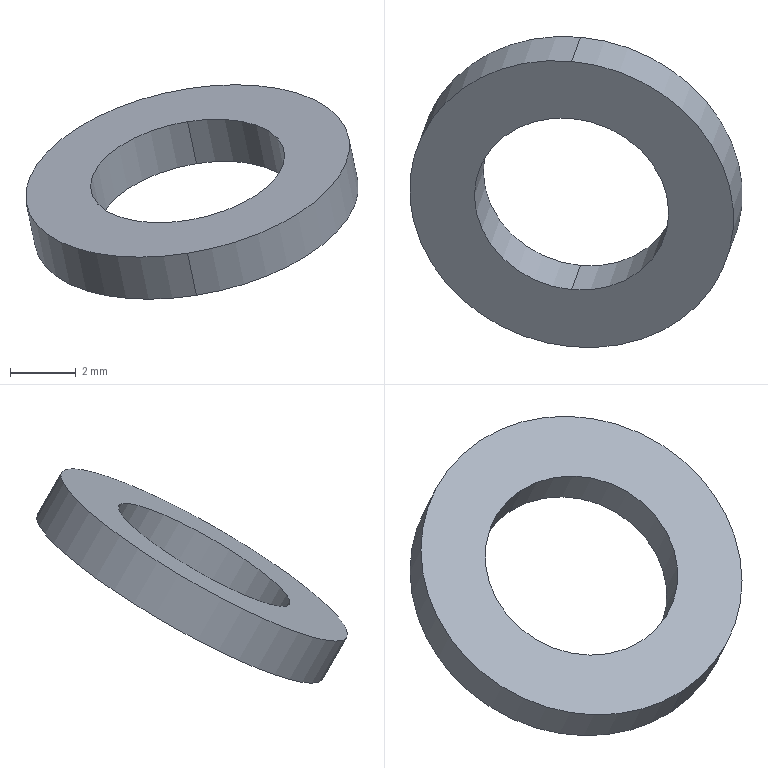Part | SolidWorks | features BaseBody 1 | 1 solid | 6 faces | box 10.107 x 9.444 x 6.513 mm | volume 75.398 mm3 | cylinder 4 | plane 2 | commonest cylinder face diameters 6 x2 10 x2
STEP:
#1=CARTESIAN_POINT('',(132.731,-41.441,-22.222));
#2=VERTEX_POINT('',#1);
#3=CARTESIAN_POINT('',(132.731,-36.245,-19.222));
#4=VERTEX_POINT('',#3);
#5=CARTESIAN_POINT('',(132.731,-38.843,-20.722));
#6=DIRECTION('',(-0.1792,-0.4919,0.852));
#7=DIRECTION('',(0.,0.866,0.5));
#8=AXIS2_PLACEMENT_3D('',#5,#6,#7);
#9=CIRCLE('',#8,3.);
#10=EDGE_CURVE('',#2,#4,#9,.T.);
#11=ORIENTED_EDGE('',*,*,#10,.T.);
#12=CARTESIAN_POINT('',(133.,-35.507,-20.5));
#13=VERTEX_POINT('',#12);
#14=CARTESIAN_POINT('',(132.731,-36.245,-19.222));
#15=DIRECTION('',(0.1792,0.4919,-0.852));
#16=VECTOR('',#15,1000.);
#17=LINE('',#14,#16);
#18=EDGE_CURVE('',#4,#13,#17,.T.);
#19=ORIENTED_EDGE('',*,*,#18,.T.);
#20=CARTESIAN_POINT('',(133.,-40.703,-23.5));
#21=VERTEX_POINT('',#20);
#22=CARTESIAN_POINT('',(133.,-38.105,-22.));
#23=DIRECTION('',(-0.1792,-0.4919,0.852));
#24=DIRECTION('',(0.,0.866,0.5));
#25=AXIS2_PLACEMENT_3D('',#22,#23,#24);
#26=CIRCLE('',#25,3.);
#27=EDGE_CURVE('',#21,#13,#26,.T.);
#28=ORIENTED_EDGE('',*,*,#27,.F.);
#29=CARTESIAN_POINT('',(132.731,-41.441,-22.222));
#30=DIRECTION('',(0.1792,0.4919,-0.852));
#31=VECTOR('',#30,1000.);
#32=LINE('',#29,#31);
#33=EDGE_CURVE('',#2,#21,#32,.T.);
#34=ORIENTED_EDGE('',*,*,#33,.F.);
#35=EDGE_LOOP('',(#11,#19,#28,#34));
#36=FACE_OUTER_BOUND('',#35,.T.);
#37=CARTESIAN_POINT('',(132.731,-38.843,-20.722));
#38=DIRECTION('',(0.1792,0.4919,-0.852));
#39=DIRECTION('',(0.,-0.866,-0.5));
#40=AXIS2_PLACEMENT_3D('',#37,#38,#39);
#41=CYLINDRICAL_SURFACE('',#40,3.);
#42=ADVANCED_FACE('',(#36),#41,.F.);
#43=CARTESIAN_POINT('',(132.731,-34.513,-18.222));
#44=VERTEX_POINT('',#43);
#45=CARTESIAN_POINT('',(132.731,-43.173,-23.222));
#46=VERTEX_POINT('',#45);
#47=CARTESIAN_POINT('',(132.731,-38.843,-20.722));
#48=DIRECTION('',(-0.1792,-0.4919,0.852));
#49=DIRECTION('',(0.,0.866,0.5));
#50=AXIS2_PLACEMENT_3D('',#47,#48,#49);
#51=CIRCLE('',#50,5.);
#52=EDGE_CURVE('',#44,#46,#51,.T.);
#53=ORIENTED_EDGE('',*,*,#52,.F.);
#54=CARTESIAN_POINT('',(133.,-33.775,-19.5));
#55=VERTEX_POINT('',#54);
#56=CARTESIAN_POINT('',(132.731,-34.513,-18.222));
#57=DIRECTION('',(0.1792,0.4919,-0.852));
#58=VECTOR('',#57,1000.);
#59=LINE('',#56,#58);
#60=EDGE_CURVE('',#44,#55,#59,.T.);
#61=ORIENTED_EDGE('',*,*,#60,.T.);
#62=CARTESIAN_POINT('',(133.,-42.435,-24.5));
#63=VERTEX_POINT('',#62);
#64=CARTESIAN_POINT('',(133.,-38.105,-22.));
#65=DIRECTION('',(-0.1792,-0.4919,0.852));
#66=DIRECTION('',(0.,0.866,0.5));
#67=AXIS2_PLACEMENT_3D('',#64,#65,#66);
#68=CIRCLE('',#67,5.);
#69=EDGE_CURVE('',#55,#63,#68,.T.);
#70=ORIENTED_EDGE('',*,*,#69,.T.);
#71=CARTESIAN_POINT('',(132.731,-43.173,-23.222));
#72=DIRECTION('',(0.1792,0.4919,-0.852));
#73=VECTOR('',#72,1000.);
#74=LINE('',#71,#73);
#75=EDGE_CURVE('',#46,#63,#74,.T.);
#76=ORIENTED_EDGE('',*,*,#75,.F.);
#77=EDGE_LOOP('',(#53,#61,#70,#76));
#78=FACE_OUTER_BOUND('',#77,.T.);
#79=CARTESIAN_POINT('',(132.731,-38.843,-20.722));
#80=DIRECTION('',(0.1792,0.4919,-0.852));
#81=DIRECTION('',(0.,-0.866,-0.5));
#82=AXIS2_PLACEMENT_3D('',#79,#80,#81);
#83=CYLINDRICAL_SURFACE('',#82,5.);
#84=ADVANCED_FACE('',(#78),#83,.T.);
#85=CARTESIAN_POINT('',(132.731,-38.843,-20.722));
#86=DIRECTION('',(-0.1792,-0.4919,0.852));
#87=DIRECTION('',(0.,0.866,0.5));
#88=AXIS2_PLACEMENT_3D('',#85,#86,#87);
#89=CIRCLE('',#88,5.);
#90=EDGE_CURVE('',#46,#44,#89,.T.);
#91=ORIENTED_EDGE('',*,*,#90,.T.);
#92=ORIENTED_EDGE('',*,*,#52,.T.);
#93=EDGE_LOOP('',(#91,#92));
#94=FACE_OUTER_BOUND('',#93,.T.);
#95=ORIENTED_EDGE('',*,*,#10,.F.);
#96=CARTESIAN_POINT('',(132.731,-38.843,-20.722));
#97=DIRECTION('',(-0.1792,-0.4919,0.852));
#98=DIRECTION('',(0.,0.866,0.5));
#99=AXIS2_PLACEMENT_3D('',#96,#97,#98);
#100=CIRCLE('',#99,3.);
#101=EDGE_CURVE('',#4,#2,#100,.T.);
#102=ORIENTED_EDGE('',*,*,#101,.F.);
#103=EDGE_LOOP('',(#95,#102));
#104=FACE_BOUND('',#103,.T.);
#105=CARTESIAN_POINT('',(132.731,-38.843,-20.722));
#106=DIRECTION('',(-0.1792,-0.4919,0.852));
#107=DIRECTION('',(0.,0.866,0.5));
#108=AXIS2_PLACEMENT_3D('',#105,#106,#107);
#109=PLANE('',#108);
#110=ADVANCED_FACE('',(#94,#104),#109,.T.);
#111=CARTESIAN_POINT('',(133.,-38.105,-22.));
#112=DIRECTION('',(-0.1792,-0.4919,0.852));
#113=DIRECTION('',(0.,0.866,0.5));
#114=AXIS2_PLACEMENT_3D('',#111,#112,#113);
#115=CIRCLE('',#114,5.);
#116=EDGE_CURVE('',#63,#55,#115,.T.);
#117=ORIENTED_EDGE('',*,*,#116,.F.);
#118=ORIENTED_EDGE('',*,*,#69,.F.);
#119=EDGE_LOOP('',(#117,#118));
#120=FACE_OUTER_BOUND('',#119,.T.);
#121=ORIENTED_EDGE('',*,*,#27,.T.);
#122=CARTESIAN_POINT('',(133.,-38.105,-22.));
#123=DIRECTION('',(-0.1792,-0.4919,0.852));
#124=DIRECTION('',(0.,0.866,0.5));
#125=AXIS2_PLACEMENT_3D('',#122,#123,#124);
#126=CIRCLE('',#125,3.);
#127=EDGE_CURVE('',#13,#21,#126,.T.);
#128=ORIENTED_EDGE('',*,*,#127,.T.);
#129=EDGE_LOOP('',(#121,#128));
#130=FACE_BOUND('',#129,.T.);
#131=CARTESIAN_POINT('',(133.,-38.105,-22.));
#132=DIRECTION('',(-0.1792,-0.4919,0.852));
#133=DIRECTION('',(0.,0.866,0.5));
#134=AXIS2_PLACEMENT_3D('',#131,#132,#133);
#135=PLANE('',#134);
#136=ADVANCED_FACE('',(#120,#130),#135,.F.);
#137=ORIENTED_EDGE('',*,*,#60,.F.);
#138=ORIENTED_EDGE('',*,*,#90,.F.);
#139=ORIENTED_EDGE('',*,*,#75,.T.);
#140=ORIENTED_EDGE('',*,*,#116,.T.);
#141=EDGE_LOOP('',(#137,#138,#139,#140));
#142=FACE_OUTER_BOUND('',#141,.T.);
#143=CARTESIAN_POINT('',(132.731,-38.843,-20.722));
#144=DIRECTION('',(0.1792,0.4919,-0.852));
#145=DIRECTION('',(0.,-0.866,-0.5));
#146=AXIS2_PLACEMENT_3D('',#143,#144,#145);
#147=CYLINDRICAL_SURFACE('',#146,5.);
#148=ADVANCED_FACE('',(#142),#147,.T.);
#149=ORIENTED_EDGE('',*,*,#18,.F.);
#150=ORIENTED_EDGE('',*,*,#101,.T.);
#151=ORIENTED_EDGE('',*,*,#33,.T.);
#152=ORIENTED_EDGE('',*,*,#127,.F.);
#153=EDGE_LOOP('',(#149,#150,#151,#152));
#154=FACE_OUTER_BOUND('',#153,.T.);
#155=CARTESIAN_POINT('',(132.731,-38.843,-20.722));
#156=DIRECTION('',(0.1792,0.4919,-0.852));
#157=DIRECTION('',(0.,-0.866,-0.5));
#158=AXIS2_PLACEMENT_3D('',#155,#156,#157);
#159=CYLINDRICAL_SURFACE('',#158,3.);
#160=ADVANCED_FACE('',(#154),#159,.F.);
#161=CLOSED_SHELL('',(#42,#84,#110,#136,#148,#160));
#162=MANIFOLD_SOLID_BREP('',#161);
#163=CARTESIAN_POINT('',(0.,0.,0.));
#164=DIRECTION('',(0.,0.,1.));
#165=DIRECTION('',(1.,0.,0.));
#166=AXIS2_PLACEMENT_3D('',#163,#164,#165);
#167=(LENGTH_UNIT()NAMED_UNIT(*)SI_UNIT(.MILLI.,.METRE.));
#168=UNCERTAINTY_MEASURE_WITH_UNIT(LENGTH_MEASURE(0.00001),#167,'','');
#169=(NAMED_UNIT(*)PLANE_ANGLE_UNIT()SI_UNIT($,.RADIAN.));
#170=(NAMED_UNIT(*)SI_UNIT($,.STERADIAN.)SOLID_ANGLE_UNIT());
#171=(GEOMETRIC_REPRESENTATION_CONTEXT(3)GLOBAL_UNCERTAINTY_ASSIGNED_CONTEXT((#168))GLOBAL_UNIT_ASSIGNED_CONTEXT((#167,#169,#170))REPRESENTATION_CONTEXT('',''));
#172=ADVANCED_BREP_SHAPE_REPRESENTATION('',(#162,#166),#171);